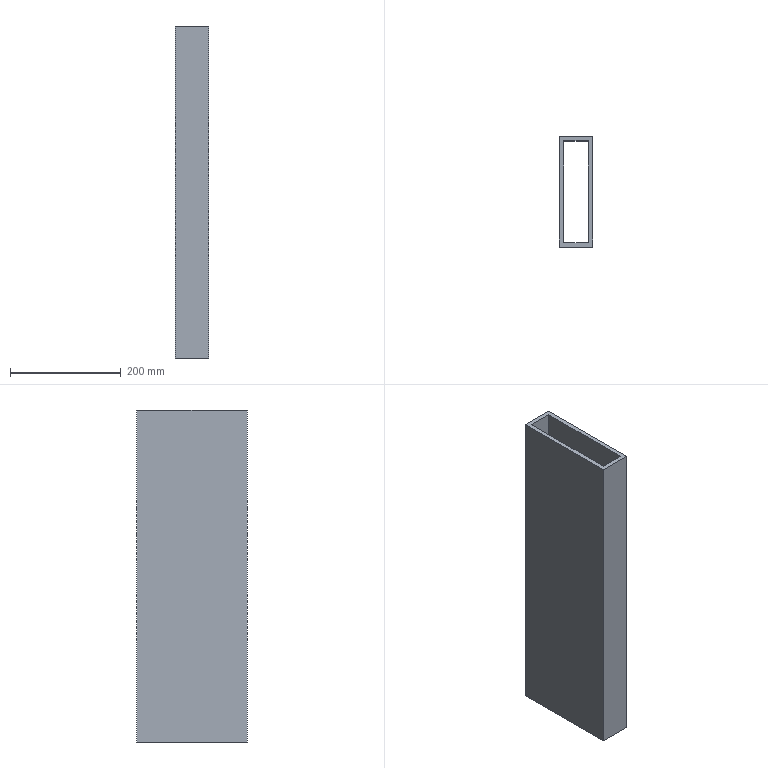Part | SolidWorks | features BaseBody 1 | 1 solid | 10 faces | box 60 x 200 x 600 mm | volume 2342400 mm3 | plane 10
STEP:
#1=CARTESIAN_POINT('',(-30.,100.,-300.));
#2=VERTEX_POINT('',#1);
#3=CARTESIAN_POINT('',(-30.,100.,300.));
#4=VERTEX_POINT('',#3);
#5=CARTESIAN_POINT('',(-30.,100.,-300.));
#6=DIRECTION('',(0.,0.,1.));
#7=VECTOR('',#6,1000.);
#8=LINE('',#5,#7);
#9=EDGE_CURVE('',#2,#4,#8,.T.);
#10=ORIENTED_EDGE('',*,*,#9,.F.);
#11=CARTESIAN_POINT('',(-30.,-100.,-300.));
#12=VERTEX_POINT('',#11);
#13=CARTESIAN_POINT('',(-30.,-100.,-300.));
#14=DIRECTION('',(0.,1.,0.));
#15=VECTOR('',#14,1000.);
#16=LINE('',#13,#15);
#17=EDGE_CURVE('',#12,#2,#16,.T.);
#18=ORIENTED_EDGE('',*,*,#17,.F.);
#19=CARTESIAN_POINT('',(-30.,-100.,300.));
#20=VERTEX_POINT('',#19);
#21=CARTESIAN_POINT('',(-30.,-100.,-300.));
#22=DIRECTION('',(0.,0.,-1.));
#23=VECTOR('',#22,1000.);
#24=LINE('',#21,#23);
#25=EDGE_CURVE('',#20,#12,#24,.T.);
#26=ORIENTED_EDGE('',*,*,#25,.F.);
#27=CARTESIAN_POINT('',(-30.,-100.,300.));
#28=DIRECTION('',(0.,-1.,0.));
#29=VECTOR('',#28,1000.);
#30=LINE('',#27,#29);
#31=EDGE_CURVE('',#4,#20,#30,.T.);
#32=ORIENTED_EDGE('',*,*,#31,.F.);
#33=EDGE_LOOP('',(#10,#18,#26,#32));
#34=FACE_OUTER_BOUND('',#33,.T.);
#35=CARTESIAN_POINT('',(-30.,-100.,-300.));
#36=DIRECTION('',(1.,0.,0.));
#37=DIRECTION('',(0.,0.,-1.));
#38=AXIS2_PLACEMENT_3D('',#35,#36,#37);
#39=PLANE('',#38);
#40=ADVANCED_FACE('',(#34),#39,.F.);
#41=CARTESIAN_POINT('',(-22.,92.,300.));
#42=VERTEX_POINT('',#41);
#43=CARTESIAN_POINT('',(22.,92.,300.));
#44=VERTEX_POINT('',#43);
#45=CARTESIAN_POINT('',(-30.,92.,300.));
#46=DIRECTION('',(1.,0.,0.));
#47=VECTOR('',#46,1000.);
#48=LINE('',#45,#47);
#49=EDGE_CURVE('',#42,#44,#48,.T.);
#50=ORIENTED_EDGE('',*,*,#49,.T.);
#51=CARTESIAN_POINT('',(22.,-92.,300.));
#52=VERTEX_POINT('',#51);
#53=CARTESIAN_POINT('',(22.,-100.,300.));
#54=DIRECTION('',(0.,-1.,0.));
#55=VECTOR('',#54,1000.);
#56=LINE('',#53,#55);
#57=EDGE_CURVE('',#44,#52,#56,.T.);
#58=ORIENTED_EDGE('',*,*,#57,.T.);
#59=CARTESIAN_POINT('',(-22.,-92.,300.));
#60=VERTEX_POINT('',#59);
#61=CARTESIAN_POINT('',(-30.,-92.,300.));
#62=DIRECTION('',(-1.,0.,0.));
#63=VECTOR('',#62,1000.);
#64=LINE('',#61,#63);
#65=EDGE_CURVE('',#52,#60,#64,.T.);
#66=ORIENTED_EDGE('',*,*,#65,.T.);
#67=CARTESIAN_POINT('',(-22.,-100.,300.));
#68=DIRECTION('',(0.,1.,0.));
#69=VECTOR('',#68,1000.);
#70=LINE('',#67,#69);
#71=EDGE_CURVE('',#60,#42,#70,.T.);
#72=ORIENTED_EDGE('',*,*,#71,.T.);
#73=EDGE_LOOP('',(#50,#58,#66,#72));
#74=FACE_BOUND('',#73,.T.);
#75=CARTESIAN_POINT('',(30.,-100.,300.));
#76=VERTEX_POINT('',#75);
#77=CARTESIAN_POINT('',(30.,100.,300.));
#78=VERTEX_POINT('',#77);
#79=CARTESIAN_POINT('',(30.,-100.,300.));
#80=DIRECTION('',(0.,1.,0.));
#81=VECTOR('',#80,1000.);
#82=LINE('',#79,#81);
#83=EDGE_CURVE('',#76,#78,#82,.T.);
#84=ORIENTED_EDGE('',*,*,#83,.T.);
#85=CARTESIAN_POINT('',(-30.,100.,300.));
#86=DIRECTION('',(-1.,0.,0.));
#87=VECTOR('',#86,1000.);
#88=LINE('',#85,#87);
#89=EDGE_CURVE('',#78,#4,#88,.T.);
#90=ORIENTED_EDGE('',*,*,#89,.T.);
#91=ORIENTED_EDGE('',*,*,#31,.T.);
#92=CARTESIAN_POINT('',(-30.,-100.,300.));
#93=DIRECTION('',(1.,0.,0.));
#94=VECTOR('',#93,1000.);
#95=LINE('',#92,#94);
#96=EDGE_CURVE('',#20,#76,#95,.T.);
#97=ORIENTED_EDGE('',*,*,#96,.T.);
#98=EDGE_LOOP('',(#84,#90,#91,#97));
#99=FACE_OUTER_BOUND('',#98,.T.);
#100=CARTESIAN_POINT('',(-30.,-100.,300.));
#101=DIRECTION('',(0.,0.,1.));
#102=DIRECTION('',(1.,0.,0.));
#103=AXIS2_PLACEMENT_3D('',#100,#101,#102);
#104=PLANE('',#103);
#105=ADVANCED_FACE('',(#74,#99),#104,.T.);
#106=ORIENTED_EDGE('',*,*,#89,.F.);
#107=CARTESIAN_POINT('',(30.,100.,-300.));
#108=VERTEX_POINT('',#107);
#109=CARTESIAN_POINT('',(30.,100.,-300.));
#110=DIRECTION('',(0.,0.,-1.));
#111=VECTOR('',#110,1000.);
#112=LINE('',#109,#111);
#113=EDGE_CURVE('',#78,#108,#112,.T.);
#114=ORIENTED_EDGE('',*,*,#113,.T.);
#115=CARTESIAN_POINT('',(-30.,100.,-300.));
#116=DIRECTION('',(-1.,0.,0.));
#117=VECTOR('',#116,1000.);
#118=LINE('',#115,#117);
#119=EDGE_CURVE('',#108,#2,#118,.T.);
#120=ORIENTED_EDGE('',*,*,#119,.T.);
#121=ORIENTED_EDGE('',*,*,#9,.T.);
#122=EDGE_LOOP('',(#106,#114,#120,#121));
#123=FACE_OUTER_BOUND('',#122,.T.);
#124=CARTESIAN_POINT('',(-30.,100.,-300.));
#125=DIRECTION('',(0.,1.,0.));
#126=DIRECTION('',(0.,0.,1.));
#127=AXIS2_PLACEMENT_3D('',#124,#125,#126);
#128=PLANE('',#127);
#129=ADVANCED_FACE('',(#123),#128,.T.);
#130=CARTESIAN_POINT('',(-22.,92.,-300.));
#131=VERTEX_POINT('',#130);
#132=CARTESIAN_POINT('',(22.,92.,-300.));
#133=VERTEX_POINT('',#132);
#134=CARTESIAN_POINT('',(-30.,92.,-300.));
#135=DIRECTION('',(1.,0.,0.));
#136=VECTOR('',#135,1000.);
#137=LINE('',#134,#136);
#138=EDGE_CURVE('',#131,#133,#137,.T.);
#139=ORIENTED_EDGE('',*,*,#138,.F.);
#140=CARTESIAN_POINT('',(-22.,-92.,-300.));
#141=VERTEX_POINT('',#140);
#142=CARTESIAN_POINT('',(-22.,-100.,-300.));
#143=DIRECTION('',(0.,1.,0.));
#144=VECTOR('',#143,1000.);
#145=LINE('',#142,#144);
#146=EDGE_CURVE('',#141,#131,#145,.T.);
#147=ORIENTED_EDGE('',*,*,#146,.F.);
#148=CARTESIAN_POINT('',(22.,-92.,-300.));
#149=VERTEX_POINT('',#148);
#150=CARTESIAN_POINT('',(-30.,-92.,-300.));
#151=DIRECTION('',(-1.,0.,0.));
#152=VECTOR('',#151,1000.);
#153=LINE('',#150,#152);
#154=EDGE_CURVE('',#149,#141,#153,.T.);
#155=ORIENTED_EDGE('',*,*,#154,.F.);
#156=CARTESIAN_POINT('',(22.,-100.,-300.));
#157=DIRECTION('',(0.,-1.,0.));
#158=VECTOR('',#157,1000.);
#159=LINE('',#156,#158);
#160=EDGE_CURVE('',#133,#149,#159,.T.);
#161=ORIENTED_EDGE('',*,*,#160,.F.);
#162=EDGE_LOOP('',(#139,#147,#155,#161));
#163=FACE_BOUND('',#162,.T.);
#164=CARTESIAN_POINT('',(30.,-100.,-300.));
#165=VERTEX_POINT('',#164);
#166=CARTESIAN_POINT('',(30.,-100.,-300.));
#167=DIRECTION('',(0.,1.,0.));
#168=VECTOR('',#167,1000.);
#169=LINE('',#166,#168);
#170=EDGE_CURVE('',#165,#108,#169,.T.);
#171=ORIENTED_EDGE('',*,*,#170,.F.);
#172=CARTESIAN_POINT('',(-30.,-100.,-300.));
#173=DIRECTION('',(1.,0.,0.));
#174=VECTOR('',#173,1000.);
#175=LINE('',#172,#174);
#176=EDGE_CURVE('',#12,#165,#175,.T.);
#177=ORIENTED_EDGE('',*,*,#176,.F.);
#178=ORIENTED_EDGE('',*,*,#17,.T.);
#179=ORIENTED_EDGE('',*,*,#119,.F.);
#180=EDGE_LOOP('',(#171,#177,#178,#179));
#181=FACE_OUTER_BOUND('',#180,.T.);
#182=CARTESIAN_POINT('',(-30.,-100.,-300.));
#183=DIRECTION('',(0.,0.,1.));
#184=DIRECTION('',(1.,0.,0.));
#185=AXIS2_PLACEMENT_3D('',#182,#183,#184);
#186=PLANE('',#185);
#187=ADVANCED_FACE('',(#163,#181),#186,.F.);
#188=ORIENTED_EDGE('',*,*,#96,.F.);
#189=ORIENTED_EDGE('',*,*,#25,.T.);
#190=ORIENTED_EDGE('',*,*,#176,.T.);
#191=CARTESIAN_POINT('',(30.,-100.,-300.));
#192=DIRECTION('',(0.,0.,-1.));
#193=VECTOR('',#192,1000.);
#194=LINE('',#191,#193);
#195=EDGE_CURVE('',#76,#165,#194,.T.);
#196=ORIENTED_EDGE('',*,*,#195,.F.);
#197=EDGE_LOOP('',(#188,#189,#190,#196));
#198=FACE_OUTER_BOUND('',#197,.T.);
#199=CARTESIAN_POINT('',(-30.,-100.,-300.));
#200=DIRECTION('',(0.,1.,0.));
#201=DIRECTION('',(0.,0.,1.));
#202=AXIS2_PLACEMENT_3D('',#199,#200,#201);
#203=PLANE('',#202);
#204=ADVANCED_FACE('',(#198),#203,.F.);
#205=CARTESIAN_POINT('',(22.,92.,-301.));
#206=DIRECTION('',(0.,0.,1.));
#207=VECTOR('',#206,1000.);
#208=LINE('',#205,#207);
#209=EDGE_CURVE('',#133,#44,#208,.T.);
#210=ORIENTED_EDGE('',*,*,#209,.F.);
#211=ORIENTED_EDGE('',*,*,#160,.T.);
#212=CARTESIAN_POINT('',(22.,-92.,-301.));
#213=DIRECTION('',(0.,0.,-1.));
#214=VECTOR('',#213,1000.);
#215=LINE('',#212,#214);
#216=EDGE_CURVE('',#52,#149,#215,.T.);
#217=ORIENTED_EDGE('',*,*,#216,.F.);
#218=ORIENTED_EDGE('',*,*,#57,.F.);
#219=EDGE_LOOP('',(#210,#211,#217,#218));
#220=FACE_OUTER_BOUND('',#219,.T.);
#221=CARTESIAN_POINT('',(22.,-92.,-301.));
#222=DIRECTION('',(1.,0.,0.));
#223=DIRECTION('',(0.,0.,-1.));
#224=AXIS2_PLACEMENT_3D('',#221,#222,#223);
#225=PLANE('',#224);
#226=ADVANCED_FACE('',(#220),#225,.F.);
#227=CARTESIAN_POINT('',(-22.,92.,-301.));
#228=DIRECTION('',(0.,0.,1.));
#229=VECTOR('',#228,1000.);
#230=LINE('',#227,#229);
#231=EDGE_CURVE('',#131,#42,#230,.T.);
#232=ORIENTED_EDGE('',*,*,#231,.F.);
#233=ORIENTED_EDGE('',*,*,#138,.T.);
#234=ORIENTED_EDGE('',*,*,#209,.T.);
#235=ORIENTED_EDGE('',*,*,#49,.F.);
#236=EDGE_LOOP('',(#232,#233,#234,#235));
#237=FACE_OUTER_BOUND('',#236,.T.);
#238=CARTESIAN_POINT('',(-22.,92.,-301.));
#239=DIRECTION('',(0.,1.,0.));
#240=DIRECTION('',(0.,0.,1.));
#241=AXIS2_PLACEMENT_3D('',#238,#239,#240);
#242=PLANE('',#241);
#243=ADVANCED_FACE('',(#237),#242,.F.);
#244=ORIENTED_EDGE('',*,*,#231,.T.);
#245=ORIENTED_EDGE('',*,*,#71,.F.);
#246=CARTESIAN_POINT('',(-22.,-92.,-301.));
#247=DIRECTION('',(0.,0.,-1.));
#248=VECTOR('',#247,1000.);
#249=LINE('',#246,#248);
#250=EDGE_CURVE('',#60,#141,#249,.T.);
#251=ORIENTED_EDGE('',*,*,#250,.T.);
#252=ORIENTED_EDGE('',*,*,#146,.T.);
#253=EDGE_LOOP('',(#244,#245,#251,#252));
#254=FACE_OUTER_BOUND('',#253,.T.);
#255=CARTESIAN_POINT('',(-22.,-92.,-301.));
#256=DIRECTION('',(1.,0.,0.));
#257=DIRECTION('',(0.,0.,-1.));
#258=AXIS2_PLACEMENT_3D('',#255,#256,#257);
#259=PLANE('',#258);
#260=ADVANCED_FACE('',(#254),#259,.T.);
#261=ORIENTED_EDGE('',*,*,#250,.F.);
#262=ORIENTED_EDGE('',*,*,#65,.F.);
#263=ORIENTED_EDGE('',*,*,#216,.T.);
#264=ORIENTED_EDGE('',*,*,#154,.T.);
#265=EDGE_LOOP('',(#261,#262,#263,#264));
#266=FACE_OUTER_BOUND('',#265,.T.);
#267=CARTESIAN_POINT('',(-22.,-92.,-301.));
#268=DIRECTION('',(0.,1.,0.));
#269=DIRECTION('',(0.,0.,1.));
#270=AXIS2_PLACEMENT_3D('',#267,#268,#269);
#271=PLANE('',#270);
#272=ADVANCED_FACE('',(#266),#271,.T.);
#273=ORIENTED_EDGE('',*,*,#113,.F.);
#274=ORIENTED_EDGE('',*,*,#83,.F.);
#275=ORIENTED_EDGE('',*,*,#195,.T.);
#276=ORIENTED_EDGE('',*,*,#170,.T.);
#277=EDGE_LOOP('',(#273,#274,#275,#276));
#278=FACE_OUTER_BOUND('',#277,.T.);
#279=CARTESIAN_POINT('',(30.,-100.,-300.));
#280=DIRECTION('',(1.,0.,0.));
#281=DIRECTION('',(0.,0.,-1.));
#282=AXIS2_PLACEMENT_3D('',#279,#280,#281);
#283=PLANE('',#282);
#284=ADVANCED_FACE('',(#278),#283,.T.);
#285=CLOSED_SHELL('',(#40,#105,#129,#187,#204,#226,#243,#260,#272,#284));
#286=MANIFOLD_SOLID_BREP('',#285);
#287=CARTESIAN_POINT('',(0.,0.,0.));
#288=DIRECTION('',(0.,0.,1.));
#289=DIRECTION('',(1.,0.,0.));
#290=AXIS2_PLACEMENT_3D('',#287,#288,#289);
#291=(LENGTH_UNIT()NAMED_UNIT(*)SI_UNIT(.MILLI.,.METRE.));
#292=UNCERTAINTY_MEASURE_WITH_UNIT(LENGTH_MEASURE(0.00001),#291,'','');
#293=(NAMED_UNIT(*)PLANE_ANGLE_UNIT()SI_UNIT($,.RADIAN.));
#294=(NAMED_UNIT(*)SI_UNIT($,.STERADIAN.)SOLID_ANGLE_UNIT());
#295=(GEOMETRIC_REPRESENTATION_CONTEXT(3)GLOBAL_UNCERTAINTY_ASSIGNED_CONTEXT((#292))GLOBAL_UNIT_ASSIGNED_CONTEXT((#291,#293,#294))REPRESENTATION_CONTEXT('',''));
#296=ADVANCED_BREP_SHAPE_REPRESENTATION('',(#286,#290),#295);